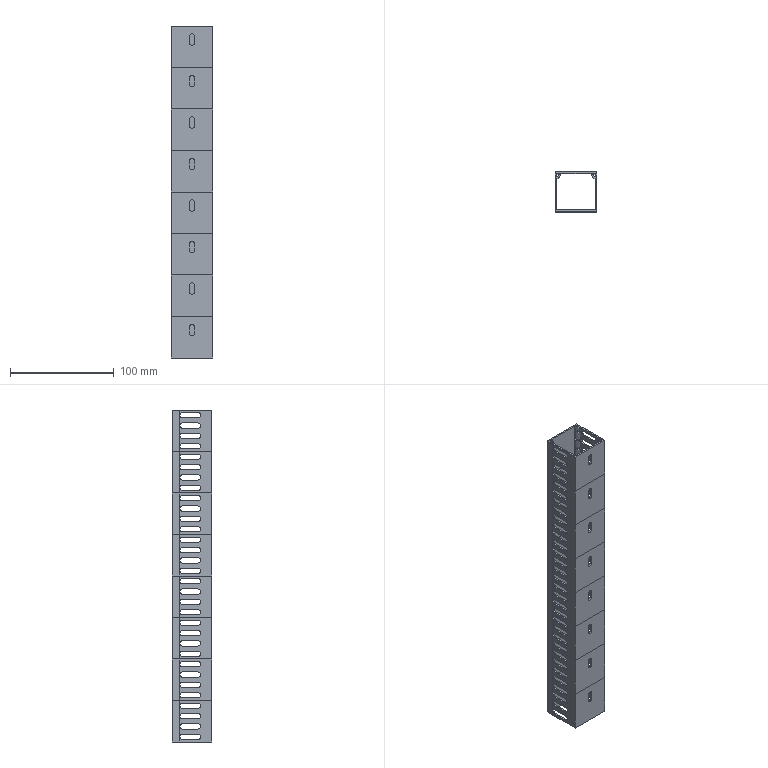Part | STEP file | 16 solids | 1336 faces | box 40 x 38.5 x 320 mm | volume 73088 mm3 | plane 688 | cylinder 648 | commonest cylinder face diameters 5 x216 1 x136 2 x120 24 x96 26 x80